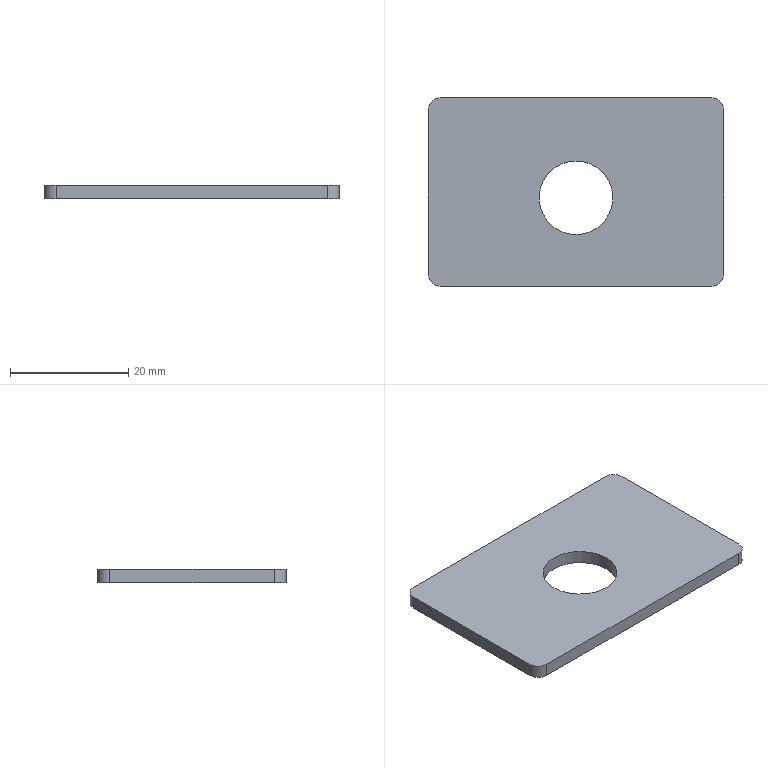Part | SolidWorks | features FlatPattern 1, SMBaseFlange 1, SheetMetal 1 | 1 solid | 12 faces | box 50 x 31.95 x 2.3 mm | volume 3384 mm3 | cylinder 6 | plane 6 | commonest cylinder face diameters 4 x4 12.5 x2
STEP:
#1=CARTESIAN_POINT('',(-6.25,15.,2.3));
#2=VERTEX_POINT('',#1);
#3=CARTESIAN_POINT('',(6.25,15.,2.3));
#4=VERTEX_POINT('',#3);
#5=CARTESIAN_POINT('',(0.,15.,2.3));
#6=DIRECTION('',(0.,0.,1.));
#7=DIRECTION('',(1.,0.,0.));
#8=AXIS2_PLACEMENT_3D('',#5,#6,#7);
#9=CIRCLE('',#8,6.25);
#10=EDGE_CURVE('',#2,#4,#9,.T.);
#11=ORIENTED_EDGE('',*,*,#10,.T.);
#12=CARTESIAN_POINT('',(6.25,15.,0.));
#13=VERTEX_POINT('',#12);
#14=CARTESIAN_POINT('',(6.25,15.,2.3));
#15=DIRECTION('',(0.,0.,-1.));
#16=VECTOR('',#15,1000.);
#17=LINE('',#14,#16);
#18=EDGE_CURVE('',#4,#13,#17,.T.);
#19=ORIENTED_EDGE('',*,*,#18,.T.);
#20=CARTESIAN_POINT('',(-6.25,15.,0.));
#21=VERTEX_POINT('',#20);
#22=CARTESIAN_POINT('',(0.,15.,0.));
#23=DIRECTION('',(0.,0.,1.));
#24=DIRECTION('',(1.,0.,0.));
#25=AXIS2_PLACEMENT_3D('',#22,#23,#24);
#26=CIRCLE('',#25,6.25);
#27=EDGE_CURVE('',#21,#13,#26,.T.);
#28=ORIENTED_EDGE('',*,*,#27,.F.);
#29=CARTESIAN_POINT('',(-6.25,15.,2.3));
#30=DIRECTION('',(0.,0.,-1.));
#31=VECTOR('',#30,1000.);
#32=LINE('',#29,#31);
#33=EDGE_CURVE('',#2,#21,#32,.T.);
#34=ORIENTED_EDGE('',*,*,#33,.F.);
#35=EDGE_LOOP('',(#11,#19,#28,#34));
#36=FACE_OUTER_BOUND('',#35,.T.);
#37=CARTESIAN_POINT('',(0.,15.,2.3));
#38=DIRECTION('',(0.,0.,-1.));
#39=DIRECTION('',(-1.,0.,0.));
#40=AXIS2_PLACEMENT_3D('',#37,#38,#39);
#41=CYLINDRICAL_SURFACE('',#40,6.25);
#42=ADVANCED_FACE('',(#36),#41,.F.);
#43=CARTESIAN_POINT('',(23.,0.,2.3));
#44=VERTEX_POINT('',#43);
#45=CARTESIAN_POINT('',(25.,2.,2.3));
#46=VERTEX_POINT('',#45);
#47=CARTESIAN_POINT('',(23.,2.,2.3));
#48=DIRECTION('',(0.,0.,1.));
#49=DIRECTION('',(1.,0.,0.));
#50=AXIS2_PLACEMENT_3D('',#47,#48,#49);
#51=CIRCLE('',#50,2.);
#52=EDGE_CURVE('',#44,#46,#51,.T.);
#53=ORIENTED_EDGE('',*,*,#52,.T.);
#54=CARTESIAN_POINT('',(25.,29.95,2.3));
#55=VERTEX_POINT('',#54);
#56=CARTESIAN_POINT('',(25.,2.,2.3));
#57=DIRECTION('',(0.,1.,0.));
#58=VECTOR('',#57,1000.);
#59=LINE('',#56,#58);
#60=EDGE_CURVE('',#46,#55,#59,.T.);
#61=ORIENTED_EDGE('',*,*,#60,.T.);
#62=CARTESIAN_POINT('',(23.,31.95,2.3));
#63=VERTEX_POINT('',#62);
#64=CARTESIAN_POINT('',(23.,29.95,2.3));
#65=DIRECTION('',(0.,0.,1.));
#66=DIRECTION('',(1.,0.,0.));
#67=AXIS2_PLACEMENT_3D('',#64,#65,#66);
#68=CIRCLE('',#67,2.);
#69=EDGE_CURVE('',#55,#63,#68,.T.);
#70=ORIENTED_EDGE('',*,*,#69,.T.);
#71=CARTESIAN_POINT('',(-23.,31.95,2.3));
#72=VERTEX_POINT('',#71);
#73=CARTESIAN_POINT('',(23.,31.95,2.3));
#74=DIRECTION('',(-1.,0.,0.));
#75=VECTOR('',#74,1000.);
#76=LINE('',#73,#75);
#77=EDGE_CURVE('',#63,#72,#76,.T.);
#78=ORIENTED_EDGE('',*,*,#77,.T.);
#79=CARTESIAN_POINT('',(-25.,29.95,2.3));
#80=VERTEX_POINT('',#79);
#81=CARTESIAN_POINT('',(-23.,29.95,2.3));
#82=DIRECTION('',(0.,0.,1.));
#83=DIRECTION('',(1.,0.,0.));
#84=AXIS2_PLACEMENT_3D('',#81,#82,#83);
#85=CIRCLE('',#84,2.);
#86=EDGE_CURVE('',#72,#80,#85,.T.);
#87=ORIENTED_EDGE('',*,*,#86,.T.);
#88=CARTESIAN_POINT('',(-25.,2.,2.3));
#89=VERTEX_POINT('',#88);
#90=CARTESIAN_POINT('',(-25.,2.,2.3));
#91=DIRECTION('',(0.,-1.,0.));
#92=VECTOR('',#91,1000.);
#93=LINE('',#90,#92);
#94=EDGE_CURVE('',#80,#89,#93,.T.);
#95=ORIENTED_EDGE('',*,*,#94,.T.);
#96=CARTESIAN_POINT('',(-23.,0.,2.3));
#97=VERTEX_POINT('',#96);
#98=CARTESIAN_POINT('',(-23.,2.,2.3));
#99=DIRECTION('',(0.,0.,1.));
#100=DIRECTION('',(-1.,0.,0.));
#101=AXIS2_PLACEMENT_3D('',#98,#99,#100);
#102=CIRCLE('',#101,2.);
#103=EDGE_CURVE('',#89,#97,#102,.T.);
#104=ORIENTED_EDGE('',*,*,#103,.T.);
#105=CARTESIAN_POINT('',(23.,0.,2.3));
#106=DIRECTION('',(1.,0.,0.));
#107=VECTOR('',#106,1000.);
#108=LINE('',#105,#107);
#109=EDGE_CURVE('',#97,#44,#108,.T.);
#110=ORIENTED_EDGE('',*,*,#109,.T.);
#111=EDGE_LOOP('',(#53,#61,#70,#78,#87,#95,#104,#110));
#112=FACE_OUTER_BOUND('',#111,.T.);
#113=ORIENTED_EDGE('',*,*,#10,.F.);
#114=CARTESIAN_POINT('',(0.,15.,2.3));
#115=DIRECTION('',(0.,0.,1.));
#116=DIRECTION('',(1.,0.,0.));
#117=AXIS2_PLACEMENT_3D('',#114,#115,#116);
#118=CIRCLE('',#117,6.25);
#119=EDGE_CURVE('',#4,#2,#118,.T.);
#120=ORIENTED_EDGE('',*,*,#119,.F.);
#121=EDGE_LOOP('',(#113,#120));
#122=FACE_BOUND('',#121,.T.);
#123=CARTESIAN_POINT('',(23.,2.,2.3));
#124=DIRECTION('',(0.,0.,1.));
#125=DIRECTION('',(1.,0.,0.));
#126=AXIS2_PLACEMENT_3D('',#123,#124,#125);
#127=PLANE('',#126);
#128=ADVANCED_FACE('',(#112,#122),#127,.T.);
#129=CARTESIAN_POINT('',(23.,0.,0.));
#130=VERTEX_POINT('',#129);
#131=CARTESIAN_POINT('',(25.,2.,0.));
#132=VERTEX_POINT('',#131);
#133=CARTESIAN_POINT('',(23.,2.,0.));
#134=DIRECTION('',(0.,0.,1.));
#135=DIRECTION('',(1.,0.,0.));
#136=AXIS2_PLACEMENT_3D('',#133,#134,#135);
#137=CIRCLE('',#136,2.);
#138=EDGE_CURVE('',#130,#132,#137,.T.);
#139=ORIENTED_EDGE('',*,*,#138,.F.);
#140=CARTESIAN_POINT('',(-23.,0.,0.));
#141=VERTEX_POINT('',#140);
#142=CARTESIAN_POINT('',(23.,0.,0.));
#143=DIRECTION('',(1.,0.,0.));
#144=VECTOR('',#143,1000.);
#145=LINE('',#142,#144);
#146=EDGE_CURVE('',#141,#130,#145,.T.);
#147=ORIENTED_EDGE('',*,*,#146,.F.);
#148=CARTESIAN_POINT('',(-25.,2.,0.));
#149=VERTEX_POINT('',#148);
#150=CARTESIAN_POINT('',(-23.,2.,0.));
#151=DIRECTION('',(0.,0.,1.));
#152=DIRECTION('',(-1.,0.,0.));
#153=AXIS2_PLACEMENT_3D('',#150,#151,#152);
#154=CIRCLE('',#153,2.);
#155=EDGE_CURVE('',#149,#141,#154,.T.);
#156=ORIENTED_EDGE('',*,*,#155,.F.);
#157=CARTESIAN_POINT('',(-25.,29.95,0.));
#158=VERTEX_POINT('',#157);
#159=CARTESIAN_POINT('',(-25.,2.,0.));
#160=DIRECTION('',(0.,-1.,0.));
#161=VECTOR('',#160,1000.);
#162=LINE('',#159,#161);
#163=EDGE_CURVE('',#158,#149,#162,.T.);
#164=ORIENTED_EDGE('',*,*,#163,.F.);
#165=CARTESIAN_POINT('',(-23.,31.95,0.));
#166=VERTEX_POINT('',#165);
#167=CARTESIAN_POINT('',(-23.,29.95,0.));
#168=DIRECTION('',(0.,0.,1.));
#169=DIRECTION('',(1.,0.,0.));
#170=AXIS2_PLACEMENT_3D('',#167,#168,#169);
#171=CIRCLE('',#170,2.);
#172=EDGE_CURVE('',#166,#158,#171,.T.);
#173=ORIENTED_EDGE('',*,*,#172,.F.);
#174=CARTESIAN_POINT('',(23.,31.95,0.));
#175=VERTEX_POINT('',#174);
#176=CARTESIAN_POINT('',(23.,31.95,0.));
#177=DIRECTION('',(-1.,0.,0.));
#178=VECTOR('',#177,1000.);
#179=LINE('',#176,#178);
#180=EDGE_CURVE('',#175,#166,#179,.T.);
#181=ORIENTED_EDGE('',*,*,#180,.F.);
#182=CARTESIAN_POINT('',(25.,29.95,0.));
#183=VERTEX_POINT('',#182);
#184=CARTESIAN_POINT('',(23.,29.95,0.));
#185=DIRECTION('',(0.,0.,1.));
#186=DIRECTION('',(1.,0.,0.));
#187=AXIS2_PLACEMENT_3D('',#184,#185,#186);
#188=CIRCLE('',#187,2.);
#189=EDGE_CURVE('',#183,#175,#188,.T.);
#190=ORIENTED_EDGE('',*,*,#189,.F.);
#191=CARTESIAN_POINT('',(25.,2.,0.));
#192=DIRECTION('',(0.,1.,0.));
#193=VECTOR('',#192,1000.);
#194=LINE('',#191,#193);
#195=EDGE_CURVE('',#132,#183,#194,.T.);
#196=ORIENTED_EDGE('',*,*,#195,.F.);
#197=EDGE_LOOP('',(#139,#147,#156,#164,#173,#181,#190,#196));
#198=FACE_OUTER_BOUND('',#197,.T.);
#199=ORIENTED_EDGE('',*,*,#27,.T.);
#200=CARTESIAN_POINT('',(0.,15.,0.));
#201=DIRECTION('',(0.,0.,1.));
#202=DIRECTION('',(1.,0.,0.));
#203=AXIS2_PLACEMENT_3D('',#200,#201,#202);
#204=CIRCLE('',#203,6.25);
#205=EDGE_CURVE('',#13,#21,#204,.T.);
#206=ORIENTED_EDGE('',*,*,#205,.T.);
#207=EDGE_LOOP('',(#199,#206));
#208=FACE_BOUND('',#207,.T.);
#209=CARTESIAN_POINT('',(23.,2.,0.));
#210=DIRECTION('',(0.,0.,1.));
#211=DIRECTION('',(1.,0.,0.));
#212=AXIS2_PLACEMENT_3D('',#209,#210,#211);
#213=PLANE('',#212);
#214=ADVANCED_FACE('',(#198,#208),#213,.F.);
#215=ORIENTED_EDGE('',*,*,#138,.T.);
#216=CARTESIAN_POINT('',(25.,2.,2.3));
#217=DIRECTION('',(0.,0.,-1.));
#218=VECTOR('',#217,1000.);
#219=LINE('',#216,#218);
#220=EDGE_CURVE('',#46,#132,#219,.T.);
#221=ORIENTED_EDGE('',*,*,#220,.F.);
#222=ORIENTED_EDGE('',*,*,#52,.F.);
#223=CARTESIAN_POINT('',(23.,0.,2.3));
#224=DIRECTION('',(0.,0.,-1.));
#225=VECTOR('',#224,1000.);
#226=LINE('',#223,#225);
#227=EDGE_CURVE('',#44,#130,#226,.T.);
#228=ORIENTED_EDGE('',*,*,#227,.T.);
#229=EDGE_LOOP('',(#215,#221,#222,#228));
#230=FACE_OUTER_BOUND('',#229,.T.);
#231=CARTESIAN_POINT('',(23.,2.,2.3));
#232=DIRECTION('',(0.,0.,-1.));
#233=DIRECTION('',(-1.,0.,0.));
#234=AXIS2_PLACEMENT_3D('',#231,#232,#233);
#235=CYLINDRICAL_SURFACE('',#234,2.);
#236=ADVANCED_FACE('',(#230),#235,.T.);
#237=ORIENTED_EDGE('',*,*,#195,.T.);
#238=CARTESIAN_POINT('',(25.,29.95,2.3));
#239=DIRECTION('',(0.,0.,-1.));
#240=VECTOR('',#239,1000.);
#241=LINE('',#238,#240);
#242=EDGE_CURVE('',#55,#183,#241,.T.);
#243=ORIENTED_EDGE('',*,*,#242,.F.);
#244=ORIENTED_EDGE('',*,*,#60,.F.);
#245=ORIENTED_EDGE('',*,*,#220,.T.);
#246=EDGE_LOOP('',(#237,#243,#244,#245));
#247=FACE_OUTER_BOUND('',#246,.T.);
#248=CARTESIAN_POINT('',(25.,2.,2.3));
#249=DIRECTION('',(-1.,0.,0.));
#250=DIRECTION('',(0.,-1.,0.));
#251=AXIS2_PLACEMENT_3D('',#248,#249,#250);
#252=PLANE('',#251);
#253=ADVANCED_FACE('',(#247),#252,.F.);
#254=ORIENTED_EDGE('',*,*,#189,.T.);
#255=CARTESIAN_POINT('',(23.,31.95,2.3));
#256=DIRECTION('',(0.,0.,-1.));
#257=VECTOR('',#256,1000.);
#258=LINE('',#255,#257);
#259=EDGE_CURVE('',#63,#175,#258,.T.);
#260=ORIENTED_EDGE('',*,*,#259,.F.);
#261=ORIENTED_EDGE('',*,*,#69,.F.);
#262=ORIENTED_EDGE('',*,*,#242,.T.);
#263=EDGE_LOOP('',(#254,#260,#261,#262));
#264=FACE_OUTER_BOUND('',#263,.T.);
#265=CARTESIAN_POINT('',(23.,29.95,2.3));
#266=DIRECTION('',(0.,0.,-1.));
#267=DIRECTION('',(-1.,0.,0.));
#268=AXIS2_PLACEMENT_3D('',#265,#266,#267);
#269=CYLINDRICAL_SURFACE('',#268,2.);
#270=ADVANCED_FACE('',(#264),#269,.T.);
#271=ORIENTED_EDGE('',*,*,#180,.T.);
#272=CARTESIAN_POINT('',(-23.,31.95,2.3));
#273=DIRECTION('',(0.,0.,-1.));
#274=VECTOR('',#273,1000.);
#275=LINE('',#272,#274);
#276=EDGE_CURVE('',#72,#166,#275,.T.);
#277=ORIENTED_EDGE('',*,*,#276,.F.);
#278=ORIENTED_EDGE('',*,*,#77,.F.);
#279=ORIENTED_EDGE('',*,*,#259,.T.);
#280=EDGE_LOOP('',(#271,#277,#278,#279));
#281=FACE_OUTER_BOUND('',#280,.T.);
#282=CARTESIAN_POINT('',(23.,31.95,2.3));
#283=DIRECTION('',(0.,-1.,0.));
#284=DIRECTION('',(0.,0.,-1.));
#285=AXIS2_PLACEMENT_3D('',#282,#283,#284);
#286=PLANE('',#285);
#287=ADVANCED_FACE('',(#281),#286,.F.);
#288=ORIENTED_EDGE('',*,*,#172,.T.);
#289=CARTESIAN_POINT('',(-25.,29.95,2.3));
#290=DIRECTION('',(0.,0.,-1.));
#291=VECTOR('',#290,1000.);
#292=LINE('',#289,#291);
#293=EDGE_CURVE('',#80,#158,#292,.T.);
#294=ORIENTED_EDGE('',*,*,#293,.F.);
#295=ORIENTED_EDGE('',*,*,#86,.F.);
#296=ORIENTED_EDGE('',*,*,#276,.T.);
#297=EDGE_LOOP('',(#288,#294,#295,#296));
#298=FACE_OUTER_BOUND('',#297,.T.);
#299=CARTESIAN_POINT('',(-23.,29.95,2.3));
#300=DIRECTION('',(0.,0.,-1.));
#301=DIRECTION('',(-1.,0.,0.));
#302=AXIS2_PLACEMENT_3D('',#299,#300,#301);
#303=CYLINDRICAL_SURFACE('',#302,2.);
#304=ADVANCED_FACE('',(#298),#303,.T.);
#305=ORIENTED_EDGE('',*,*,#163,.T.);
#306=CARTESIAN_POINT('',(-25.,2.,2.3));
#307=DIRECTION('',(0.,0.,-1.));
#308=VECTOR('',#307,1000.);
#309=LINE('',#306,#308);
#310=EDGE_CURVE('',#89,#149,#309,.T.);
#311=ORIENTED_EDGE('',*,*,#310,.F.);
#312=ORIENTED_EDGE('',*,*,#94,.F.);
#313=ORIENTED_EDGE('',*,*,#293,.T.);
#314=EDGE_LOOP('',(#305,#311,#312,#313));
#315=FACE_OUTER_BOUND('',#314,.T.);
#316=CARTESIAN_POINT('',(-25.,2.,2.3));
#317=DIRECTION('',(1.,0.,0.));
#318=DIRECTION('',(0.,1.,0.));
#319=AXIS2_PLACEMENT_3D('',#316,#317,#318);
#320=PLANE('',#319);
#321=ADVANCED_FACE('',(#315),#320,.F.);
#322=ORIENTED_EDGE('',*,*,#155,.T.);
#323=CARTESIAN_POINT('',(-23.,0.,2.3));
#324=DIRECTION('',(0.,0.,-1.));
#325=VECTOR('',#324,1000.);
#326=LINE('',#323,#325);
#327=EDGE_CURVE('',#97,#141,#326,.T.);
#328=ORIENTED_EDGE('',*,*,#327,.F.);
#329=ORIENTED_EDGE('',*,*,#103,.F.);
#330=ORIENTED_EDGE('',*,*,#310,.T.);
#331=EDGE_LOOP('',(#322,#328,#329,#330));
#332=FACE_OUTER_BOUND('',#331,.T.);
#333=CARTESIAN_POINT('',(-23.,2.,2.3));
#334=DIRECTION('',(0.,0.,-1.));
#335=DIRECTION('',(-1.,0.,0.));
#336=AXIS2_PLACEMENT_3D('',#333,#334,#335);
#337=CYLINDRICAL_SURFACE('',#336,2.);
#338=ADVANCED_FACE('',(#332),#337,.T.);
#339=ORIENTED_EDGE('',*,*,#146,.T.);
#340=ORIENTED_EDGE('',*,*,#227,.F.);
#341=ORIENTED_EDGE('',*,*,#109,.F.);
#342=ORIENTED_EDGE('',*,*,#327,.T.);
#343=EDGE_LOOP('',(#339,#340,#341,#342));
#344=FACE_OUTER_BOUND('',#343,.T.);
#345=CARTESIAN_POINT('',(23.,0.,2.3));
#346=DIRECTION('',(0.,1.,0.));
#347=DIRECTION('',(0.,0.,1.));
#348=AXIS2_PLACEMENT_3D('',#345,#346,#347);
#349=PLANE('',#348);
#350=ADVANCED_FACE('',(#344),#349,.F.);
#351=ORIENTED_EDGE('',*,*,#18,.F.);
#352=ORIENTED_EDGE('',*,*,#119,.T.);
#353=ORIENTED_EDGE('',*,*,#33,.T.);
#354=ORIENTED_EDGE('',*,*,#205,.F.);
#355=EDGE_LOOP('',(#351,#352,#353,#354));
#356=FACE_OUTER_BOUND('',#355,.T.);
#357=CARTESIAN_POINT('',(0.,15.,2.3));
#358=DIRECTION('',(0.,0.,-1.));
#359=DIRECTION('',(-1.,0.,0.));
#360=AXIS2_PLACEMENT_3D('',#357,#358,#359);
#361=CYLINDRICAL_SURFACE('',#360,6.25);
#362=ADVANCED_FACE('',(#356),#361,.F.);
#363=CLOSED_SHELL('',(#42,#128,#214,#236,#253,#270,#287,#304,#321,#338,#350,#362));
#364=MANIFOLD_SOLID_BREP('',#363);
#365=CARTESIAN_POINT('',(0.,0.,0.));
#366=DIRECTION('',(0.,0.,1.));
#367=DIRECTION('',(1.,0.,0.));
#368=AXIS2_PLACEMENT_3D('',#365,#366,#367);
#369=(LENGTH_UNIT()NAMED_UNIT(*)SI_UNIT(.MILLI.,.METRE.));
#370=UNCERTAINTY_MEASURE_WITH_UNIT(LENGTH_MEASURE(0.00001),#369,'','');
#371=(NAMED_UNIT(*)PLANE_ANGLE_UNIT()SI_UNIT($,.RADIAN.));
#372=(NAMED_UNIT(*)SI_UNIT($,.STERADIAN.)SOLID_ANGLE_UNIT());
#373=(GEOMETRIC_REPRESENTATION_CONTEXT(3)GLOBAL_UNCERTAINTY_ASSIGNED_CONTEXT((#370))GLOBAL_UNIT_ASSIGNED_CONTEXT((#369,#371,#372))REPRESENTATION_CONTEXT('',''));
#374=ADVANCED_BREP_SHAPE_REPRESENTATION('',(#364,#368),#373);